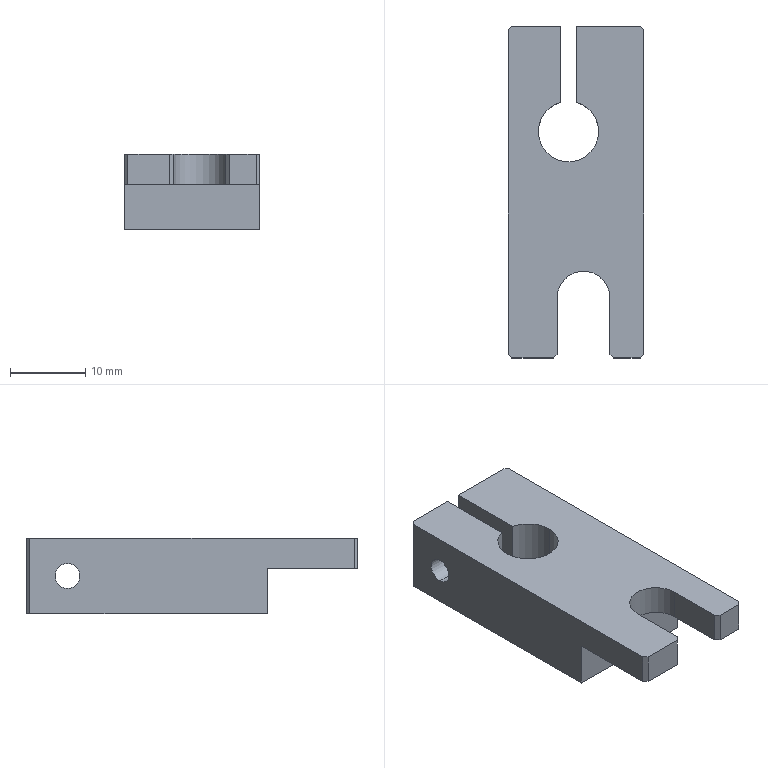Part | NX | features BREP 1 | 1 solid | 31 faces | box 18 x 44 x 10 mm | volume 5264 mm3 | plane 21 | cylinder 10 | commonest cylinder face diameters 8 x5 3.3 x2 4.8 x2 7 x1
STEP:
#1=CARTESIAN_POINT('',(6.,38.5,4.));
#2=VERTEX_POINT('',#1);
#3=CARTESIAN_POINT('',(6.,38.5,-4.));
#4=VERTEX_POINT('',#3);
#5=CARTESIAN_POINT('',(6.,38.5,0.));
#6=DIRECTION('',(1.,0.,0.));
#7=DIRECTION('',(0.,0.,-1.));
#8=AXIS2_PLACEMENT_3D('',#5,#6,#7);
#9=CIRCLE('',#8,4.);
#10=EDGE_CURVE('',#2,#4,#9,.T.);
#11=ORIENTED_EDGE('',*,*,#10,.F.);
#12=CARTESIAN_POINT('',(10.,38.5,4.));
#13=VERTEX_POINT('',#12);
#14=CARTESIAN_POINT('',(10.,38.5,4.));
#15=DIRECTION('',(1.,0.,0.));
#16=VECTOR('',#15,1000.);
#17=LINE('',#14,#16);
#18=EDGE_CURVE('',#2,#13,#17,.T.);
#19=ORIENTED_EDGE('',*,*,#18,.T.);
#20=CARTESIAN_POINT('',(10.,38.5,-4.));
#21=VERTEX_POINT('',#20);
#22=CARTESIAN_POINT('',(10.,38.5,0.));
#23=DIRECTION('',(1.,0.,0.));
#24=DIRECTION('',(0.,0.,-1.));
#25=AXIS2_PLACEMENT_3D('',#22,#23,#24);
#26=CIRCLE('',#25,4.);
#27=EDGE_CURVE('',#13,#21,#26,.T.);
#28=ORIENTED_EDGE('',*,*,#27,.T.);
#29=CARTESIAN_POINT('',(10.,38.5,-4.));
#30=DIRECTION('',(1.,0.,0.));
#31=VECTOR('',#30,1000.);
#32=LINE('',#29,#31);
#33=EDGE_CURVE('',#4,#21,#32,.T.);
#34=ORIENTED_EDGE('',*,*,#33,.F.);
#35=EDGE_LOOP('',(#11,#19,#28,#34));
#36=FACE_BOUND('',#35,.T.);
#37=CARTESIAN_POINT('',(10.,38.5,0.));
#38=DIRECTION('',(1.,0.,0.));
#39=DIRECTION('',(0.,0.,-1.));
#40=AXIS2_PLACEMENT_3D('',#37,#38,#39);
#41=CYLINDRICAL_SURFACE('',#40,4.);
#42=ADVANCED_FACE('',(#36),#41,.F.);
#43=CARTESIAN_POINT('',(1.,38.5,-2.4));
#44=VERTEX_POINT('',#43);
#45=CARTESIAN_POINT('',(1.,38.5,2.4));
#46=VERTEX_POINT('',#45);
#47=CARTESIAN_POINT('',(1.,38.5,0.));
#48=DIRECTION('',(-1.,0.,0.));
#49=DIRECTION('',(0.,0.,1.));
#50=AXIS2_PLACEMENT_3D('',#47,#48,#49);
#51=CIRCLE('',#50,2.4);
#52=EDGE_CURVE('',#44,#46,#51,.T.);
#53=ORIENTED_EDGE('',*,*,#52,.T.);
#54=CARTESIAN_POINT('',(6.,38.5,2.4));
#55=VERTEX_POINT('',#54);
#56=CARTESIAN_POINT('',(10.,38.5,2.4));
#57=DIRECTION('',(1.,0.,0.));
#58=VECTOR('',#57,1000.);
#59=LINE('',#56,#58);
#60=EDGE_CURVE('',#46,#55,#59,.T.);
#61=ORIENTED_EDGE('',*,*,#60,.T.);
#62=CARTESIAN_POINT('',(6.,38.5,-2.4));
#63=VERTEX_POINT('',#62);
#64=CARTESIAN_POINT('',(6.,38.5,0.));
#65=DIRECTION('',(1.,0.,0.));
#66=DIRECTION('',(0.,0.,-1.));
#67=AXIS2_PLACEMENT_3D('',#64,#65,#66);
#68=CIRCLE('',#67,2.4);
#69=EDGE_CURVE('',#55,#63,#68,.T.);
#70=ORIENTED_EDGE('',*,*,#69,.T.);
#71=CARTESIAN_POINT('',(10.,38.5,-2.4));
#72=DIRECTION('',(1.,0.,0.));
#73=VECTOR('',#72,1000.);
#74=LINE('',#71,#73);
#75=EDGE_CURVE('',#44,#63,#74,.T.);
#76=ORIENTED_EDGE('',*,*,#75,.F.);
#77=EDGE_LOOP('',(#53,#61,#70,#76));
#78=FACE_BOUND('',#77,.T.);
#79=CARTESIAN_POINT('',(10.,38.5,0.));
#80=DIRECTION('',(1.,0.,0.));
#81=DIRECTION('',(0.,0.,-1.));
#82=AXIS2_PLACEMENT_3D('',#79,#80,#81);
#83=CYLINDRICAL_SURFACE('',#82,2.4);
#84=ADVANCED_FACE('',(#78),#83,.F.);
#85=CARTESIAN_POINT('',(-8.,38.5,1.65));
#86=VERTEX_POINT('',#85);
#87=CARTESIAN_POINT('',(-8.,38.5,-1.65));
#88=VERTEX_POINT('',#87);
#89=CARTESIAN_POINT('',(-8.,38.5,0.));
#90=DIRECTION('',(1.,0.,0.));
#91=DIRECTION('',(0.,0.,-1.));
#92=AXIS2_PLACEMENT_3D('',#89,#90,#91);
#93=CIRCLE('',#92,1.65);
#94=EDGE_CURVE('',#86,#88,#93,.T.);
#95=ORIENTED_EDGE('',*,*,#94,.F.);
#96=CARTESIAN_POINT('',(-1.,38.5,1.65));
#97=VERTEX_POINT('',#96);
#98=CARTESIAN_POINT('',(-1.,38.5,1.65));
#99=DIRECTION('',(1.,0.,0.));
#100=VECTOR('',#99,1000.);
#101=LINE('',#98,#100);
#102=EDGE_CURVE('',#86,#97,#101,.T.);
#103=ORIENTED_EDGE('',*,*,#102,.T.);
#104=CARTESIAN_POINT('',(-1.,38.5,-1.65));
#105=VERTEX_POINT('',#104);
#106=CARTESIAN_POINT('',(-1.,38.5,0.));
#107=DIRECTION('',(1.,0.,0.));
#108=DIRECTION('',(0.,0.,-1.));
#109=AXIS2_PLACEMENT_3D('',#106,#107,#108);
#110=CIRCLE('',#109,1.65);
#111=EDGE_CURVE('',#97,#105,#110,.T.);
#112=ORIENTED_EDGE('',*,*,#111,.T.);
#113=CARTESIAN_POINT('',(-1.,38.5,-1.65));
#114=DIRECTION('',(1.,0.,0.));
#115=VECTOR('',#114,1000.);
#116=LINE('',#113,#115);
#117=EDGE_CURVE('',#88,#105,#116,.T.);
#118=ORIENTED_EDGE('',*,*,#117,.F.);
#119=EDGE_LOOP('',(#95,#103,#112,#118));
#120=FACE_BOUND('',#119,.T.);
#121=CARTESIAN_POINT('',(-1.,38.5,0.));
#122=DIRECTION('',(1.,0.,0.));
#123=DIRECTION('',(0.,0.,-1.));
#124=AXIS2_PLACEMENT_3D('',#121,#122,#123);
#125=CYLINDRICAL_SURFACE('',#124,1.65);
#126=ADVANCED_FACE('',(#120),#125,.F.);
#127=CARTESIAN_POINT('',(-4.,30.,5.));
#128=VERTEX_POINT('',#127);
#129=CARTESIAN_POINT('',(4.,30.,5.));
#130=VERTEX_POINT('',#129);
#131=CARTESIAN_POINT('',(0.,30.,5.));
#132=DIRECTION('',(0.,0.,1.));
#133=DIRECTION('',(1.,0.,0.));
#134=AXIS2_PLACEMENT_3D('',#131,#132,#133);
#135=CIRCLE('',#134,4.);
#136=EDGE_CURVE('',#128,#130,#135,.T.);
#137=ORIENTED_EDGE('',*,*,#136,.T.);
#138=CARTESIAN_POINT('',(4.,30.,-5.));
#139=VERTEX_POINT('',#138);
#140=CARTESIAN_POINT('',(4.,30.,5.));
#141=DIRECTION('',(0.,0.,-1.));
#142=VECTOR('',#141,1000.);
#143=LINE('',#140,#142);
#144=EDGE_CURVE('',#130,#139,#143,.T.);
#145=ORIENTED_EDGE('',*,*,#144,.T.);
#146=CARTESIAN_POINT('',(-4.,30.,-5.));
#147=VERTEX_POINT('',#146);
#148=CARTESIAN_POINT('',(0.,30.,-5.));
#149=DIRECTION('',(0.,0.,1.));
#150=DIRECTION('',(1.,0.,0.));
#151=AXIS2_PLACEMENT_3D('',#148,#149,#150);
#152=CIRCLE('',#151,4.);
#153=EDGE_CURVE('',#147,#139,#152,.T.);
#154=ORIENTED_EDGE('',*,*,#153,.F.);
#155=CARTESIAN_POINT('',(-4.,30.,5.));
#156=DIRECTION('',(0.,0.,-1.));
#157=VECTOR('',#156,1000.);
#158=LINE('',#155,#157);
#159=EDGE_CURVE('',#128,#147,#158,.T.);
#160=ORIENTED_EDGE('',*,*,#159,.F.);
#161=EDGE_LOOP('',(#137,#145,#154,#160));
#162=FACE_BOUND('',#161,.T.);
#163=CARTESIAN_POINT('',(0.,30.,5.));
#164=DIRECTION('',(0.,0.,-1.));
#165=DIRECTION('',(-1.,0.,0.));
#166=AXIS2_PLACEMENT_3D('',#163,#164,#165);
#167=CYLINDRICAL_SURFACE('',#166,4.);
#168=ADVANCED_FACE('',(#162),#167,.F.);
#169=CARTESIAN_POINT('',(-1.,33.873,5.));
#170=VERTEX_POINT('',#169);
#171=CARTESIAN_POINT('',(0.,30.,5.));
#172=DIRECTION('',(0.,0.,1.));
#173=DIRECTION('',(1.,0.,0.));
#174=AXIS2_PLACEMENT_3D('',#171,#172,#173);
#175=CIRCLE('',#174,4.);
#176=EDGE_CURVE('',#170,#128,#175,.T.);
#177=ORIENTED_EDGE('',*,*,#176,.T.);
#178=ORIENTED_EDGE('',*,*,#159,.T.);
#179=CARTESIAN_POINT('',(-1.,33.873,-5.));
#180=VERTEX_POINT('',#179);
#181=CARTESIAN_POINT('',(0.,30.,-5.));
#182=DIRECTION('',(0.,0.,1.));
#183=DIRECTION('',(1.,0.,0.));
#184=AXIS2_PLACEMENT_3D('',#181,#182,#183);
#185=CIRCLE('',#184,4.);
#186=EDGE_CURVE('',#180,#147,#185,.T.);
#187=ORIENTED_EDGE('',*,*,#186,.F.);
#188=CARTESIAN_POINT('',(-1.,33.873,5.));
#189=DIRECTION('',(0.,0.,1.));
#190=VECTOR('',#189,1000.);
#191=LINE('',#188,#190);
#192=EDGE_CURVE('',#180,#170,#191,.T.);
#193=ORIENTED_EDGE('',*,*,#192,.T.);
#194=EDGE_LOOP('',(#177,#178,#187,#193));
#195=FACE_BOUND('',#194,.T.);
#196=CARTESIAN_POINT('',(0.,30.,5.));
#197=DIRECTION('',(0.,0.,-1.));
#198=DIRECTION('',(-1.,0.,0.));
#199=AXIS2_PLACEMENT_3D('',#196,#197,#198);
#200=CYLINDRICAL_SURFACE('',#199,4.);
#201=ADVANCED_FACE('',(#195),#200,.F.);
#202=CARTESIAN_POINT('',(6.,0.,1.));
#203=VERTEX_POINT('',#202);
#204=CARTESIAN_POINT('',(9.5,0.,1.));
#205=VERTEX_POINT('',#204);
#206=CARTESIAN_POINT('',(-8.,0.,1.));
#207=DIRECTION('',(1.,0.,0.));
#208=VECTOR('',#207,1000.);
#209=LINE('',#206,#208);
#210=EDGE_CURVE('',#203,#205,#209,.T.);
#211=ORIENTED_EDGE('',*,*,#210,.T.);
#212=CARTESIAN_POINT('',(9.5,0.,5.));
#213=VERTEX_POINT('',#212);
#214=CARTESIAN_POINT('',(9.5,0.,5.));
#215=DIRECTION('',(0.,0.,1.));
#216=VECTOR('',#215,1000.);
#217=LINE('',#214,#216);
#218=EDGE_CURVE('',#205,#213,#217,.T.);
#219=ORIENTED_EDGE('',*,*,#218,.T.);
#220=CARTESIAN_POINT('',(6.,0.,5.));
#221=VERTEX_POINT('',#220);
#222=CARTESIAN_POINT('',(-8.,0.,5.));
#223=DIRECTION('',(1.,0.,0.));
#224=VECTOR('',#223,1000.);
#225=LINE('',#222,#224);
#226=EDGE_CURVE('',#221,#213,#225,.T.);
#227=ORIENTED_EDGE('',*,*,#226,.F.);
#228=CARTESIAN_POINT('',(6.,0.,5.));
#229=DIRECTION('',(0.,0.,-1.));
#230=VECTOR('',#229,1000.);
#231=LINE('',#228,#230);
#232=EDGE_CURVE('',#221,#203,#231,.T.);
#233=ORIENTED_EDGE('',*,*,#232,.T.);
#234=EDGE_LOOP('',(#211,#219,#227,#233));
#235=FACE_BOUND('',#234,.T.);
#236=CARTESIAN_POINT('',(-8.,0.,5.));
#237=DIRECTION('',(0.,1.,0.));
#238=DIRECTION('',(1.,0.,0.));
#239=AXIS2_PLACEMENT_3D('',#236,#237,#238);
#240=PLANE('',#239);
#241=ADVANCED_FACE('',(#235),#240,.F.);
#242=CARTESIAN_POINT('',(-1.,44.,5.));
#243=VERTEX_POINT('',#242);
#244=CARTESIAN_POINT('',(-7.5,44.,5.));
#245=VERTEX_POINT('',#244);
#246=CARTESIAN_POINT('',(10.,44.,5.));
#247=DIRECTION('',(-1.,0.,0.));
#248=VECTOR('',#247,1000.);
#249=LINE('',#246,#248);
#250=EDGE_CURVE('',#243,#245,#249,.T.);
#251=ORIENTED_EDGE('',*,*,#250,.T.);
#252=CARTESIAN_POINT('',(-8.,43.5,5.));
#253=VERTEX_POINT('',#252);
#254=CARTESIAN_POINT('',(1.25,52.75,5.));
#255=DIRECTION('',(-0.7071,-0.7071,0.));
#256=VECTOR('',#255,1000.);
#257=LINE('',#254,#256);
#258=EDGE_CURVE('',#245,#253,#257,.T.);
#259=ORIENTED_EDGE('',*,*,#258,.T.);
#260=CARTESIAN_POINT('',(-8.,0.5,5.));
#261=VERTEX_POINT('',#260);
#262=CARTESIAN_POINT('',(-8.,0.,5.));
#263=DIRECTION('',(0.,-1.,0.));
#264=VECTOR('',#263,1000.);
#265=LINE('',#262,#264);
#266=EDGE_CURVE('',#253,#261,#265,.T.);
#267=ORIENTED_EDGE('',*,*,#266,.T.);
#268=CARTESIAN_POINT('',(-7.5,0.,5.));
#269=VERTEX_POINT('',#268);
#270=CARTESIAN_POINT('',(-20.75,13.25,5.));
#271=DIRECTION('',(0.7071,-0.7071,0.));
#272=VECTOR('',#271,1000.);
#273=LINE('',#270,#272);
#274=EDGE_CURVE('',#261,#269,#273,.T.);
#275=ORIENTED_EDGE('',*,*,#274,.T.);
#276=CARTESIAN_POINT('',(-2.,0.,5.));
#277=VERTEX_POINT('',#276);
#278=CARTESIAN_POINT('',(-8.,0.,5.));
#279=DIRECTION('',(1.,0.,0.));
#280=VECTOR('',#279,1000.);
#281=LINE('',#278,#280);
#282=EDGE_CURVE('',#269,#277,#281,.T.);
#283=ORIENTED_EDGE('',*,*,#282,.T.);
#284=CARTESIAN_POINT('',(-1.5,0.5,5.));
#285=VERTEX_POINT('',#284);
#286=CARTESIAN_POINT('',(26.,28.,5.));
#287=DIRECTION('',(0.7071,0.7071,0.));
#288=VECTOR('',#287,1000.);
#289=LINE('',#286,#288);
#290=EDGE_CURVE('',#277,#285,#289,.T.);
#291=ORIENTED_EDGE('',*,*,#290,.T.);
#292=CARTESIAN_POINT('',(-1.5,8.,5.));
#293=VERTEX_POINT('',#292);
#294=CARTESIAN_POINT('',(-1.5,8.,5.));
#295=DIRECTION('',(0.,1.,0.));
#296=VECTOR('',#295,1000.);
#297=LINE('',#294,#296);
#298=EDGE_CURVE('',#285,#293,#297,.T.);
#299=ORIENTED_EDGE('',*,*,#298,.T.);
#300=CARTESIAN_POINT('',(5.5,8.,5.));
#301=VERTEX_POINT('',#300);
#302=CARTESIAN_POINT('',(2.,8.,5.));
#303=DIRECTION('',(0.,0.,-1.));
#304=DIRECTION('',(-1.,0.,0.));
#305=AXIS2_PLACEMENT_3D('',#302,#303,#304);
#306=CIRCLE('',#305,3.5);
#307=EDGE_CURVE('',#293,#301,#306,.T.);
#308=ORIENTED_EDGE('',*,*,#307,.T.);
#309=CARTESIAN_POINT('',(5.5,0.5,5.));
#310=VERTEX_POINT('',#309);
#311=CARTESIAN_POINT('',(5.5,8.,5.));
#312=DIRECTION('',(0.,-1.,0.));
#313=VECTOR('',#312,1000.);
#314=LINE('',#311,#313);
#315=EDGE_CURVE('',#301,#310,#314,.T.);
#316=ORIENTED_EDGE('',*,*,#315,.T.);
#317=CARTESIAN_POINT('',(-14.,20.,5.));
#318=DIRECTION('',(0.7071,-0.7071,0.));
#319=VECTOR('',#318,1000.);
#320=LINE('',#317,#319);
#321=EDGE_CURVE('',#310,#221,#320,.T.);
#322=ORIENTED_EDGE('',*,*,#321,.T.);
#323=ORIENTED_EDGE('',*,*,#226,.T.);
#324=CARTESIAN_POINT('',(10.,0.5,5.));
#325=VERTEX_POINT('',#324);
#326=CARTESIAN_POINT('',(31.75,22.25,5.));
#327=DIRECTION('',(0.7071,0.7071,0.));
#328=VECTOR('',#327,1000.);
#329=LINE('',#326,#328);
#330=EDGE_CURVE('',#213,#325,#329,.T.);
#331=ORIENTED_EDGE('',*,*,#330,.T.);
#332=CARTESIAN_POINT('',(10.,43.5,5.));
#333=VERTEX_POINT('',#332);
#334=CARTESIAN_POINT('',(10.,0.,5.));
#335=DIRECTION('',(0.,1.,0.));
#336=VECTOR('',#335,1000.);
#337=LINE('',#334,#336);
#338=EDGE_CURVE('',#325,#333,#337,.T.);
#339=ORIENTED_EDGE('',*,*,#338,.T.);
#340=CARTESIAN_POINT('',(9.5,44.,5.));
#341=VERTEX_POINT('',#340);
#342=CARTESIAN_POINT('',(9.75,43.75,5.));
#343=DIRECTION('',(-0.7071,0.7071,0.));
#344=VECTOR('',#343,1000.);
#345=LINE('',#342,#344);
#346=EDGE_CURVE('',#333,#341,#345,.T.);
#347=ORIENTED_EDGE('',*,*,#346,.T.);
#348=CARTESIAN_POINT('',(1.,44.,5.));
#349=VERTEX_POINT('',#348);
#350=CARTESIAN_POINT('',(10.,44.,5.));
#351=DIRECTION('',(-1.,0.,0.));
#352=VECTOR('',#351,1000.);
#353=LINE('',#350,#352);
#354=EDGE_CURVE('',#341,#349,#353,.T.);
#355=ORIENTED_EDGE('',*,*,#354,.T.);
#356=CARTESIAN_POINT('',(1.,33.873,5.));
#357=VERTEX_POINT('',#356);
#358=CARTESIAN_POINT('',(1.,44.,5.));
#359=DIRECTION('',(0.,-1.,0.));
#360=VECTOR('',#359,1000.);
#361=LINE('',#358,#360);
#362=EDGE_CURVE('',#349,#357,#361,.T.);
#363=ORIENTED_EDGE('',*,*,#362,.T.);
#364=CARTESIAN_POINT('',(0.,30.,5.));
#365=DIRECTION('',(0.,0.,1.));
#366=DIRECTION('',(1.,0.,0.));
#367=AXIS2_PLACEMENT_3D('',#364,#365,#366);
#368=CIRCLE('',#367,4.);
#369=EDGE_CURVE('',#130,#357,#368,.T.);
#370=ORIENTED_EDGE('',*,*,#369,.F.);
#371=ORIENTED_EDGE('',*,*,#136,.F.);
#372=ORIENTED_EDGE('',*,*,#176,.F.);
#373=CARTESIAN_POINT('',(-1.,44.,5.));
#374=DIRECTION('',(0.,1.,0.));
#375=VECTOR('',#374,1000.);
#376=LINE('',#373,#375);
#377=EDGE_CURVE('',#170,#243,#376,.T.);
#378=ORIENTED_EDGE('',*,*,#377,.T.);
#379=EDGE_LOOP('',(#251,#259,#267,#275,#283,#291,#299,#308,#316,#322,#323,#331,#339,#347,#355,#363,#370,#371,#372,#378));
#380=FACE_BOUND('',#379,.T.);
#381=CARTESIAN_POINT('',(10.,44.,5.));
#382=DIRECTION('',(0.,0.,1.));
#383=DIRECTION('',(1.,0.,0.));
#384=AXIS2_PLACEMENT_3D('',#381,#382,#383);
#385=PLANE('',#384);
#386=ADVANCED_FACE('',(#380),#385,.T.);
#387=CARTESIAN_POINT('',(-1.,44.,-5.));
#388=VERTEX_POINT('',#387);
#389=CARTESIAN_POINT('',(-7.5,44.,-5.));
#390=VERTEX_POINT('',#389);
#391=CARTESIAN_POINT('',(10.,44.,-5.));
#392=DIRECTION('',(-1.,0.,0.));
#393=VECTOR('',#392,1000.);
#394=LINE('',#391,#393);
#395=EDGE_CURVE('',#388,#390,#394,.T.);
#396=ORIENTED_EDGE('',*,*,#395,.T.);
#397=CARTESIAN_POINT('',(-7.5,44.,5.));
#398=DIRECTION('',(0.,0.,1.));
#399=VECTOR('',#398,1000.);
#400=LINE('',#397,#399);
#401=EDGE_CURVE('',#390,#245,#400,.T.);
#402=ORIENTED_EDGE('',*,*,#401,.T.);
#403=ORIENTED_EDGE('',*,*,#250,.F.);
#404=CARTESIAN_POINT('',(-1.,44.,6.));
#405=DIRECTION('',(0.,0.,-1.));
#406=VECTOR('',#405,1000.);
#407=LINE('',#404,#406);
#408=EDGE_CURVE('',#243,#388,#407,.T.);
#409=ORIENTED_EDGE('',*,*,#408,.T.);
#410=EDGE_LOOP('',(#396,#402,#403,#409));
#411=FACE_BOUND('',#410,.T.);
#412=CARTESIAN_POINT('',(10.,44.,5.));
#413=DIRECTION('',(0.,-1.,0.));
#414=DIRECTION('',(0.,0.,-1.));
#415=AXIS2_PLACEMENT_3D('',#412,#413,#414);
#416=PLANE('',#415);
#417=ADVANCED_FACE('',(#411),#416,.F.);
#418=ORIENTED_EDGE('',*,*,#354,.F.);
#419=CARTESIAN_POINT('',(9.5,44.,-5.));
#420=VERTEX_POINT('',#419);
#421=CARTESIAN_POINT('',(9.5,44.,5.));
#422=DIRECTION('',(0.,0.,-1.));
#423=VECTOR('',#422,1000.);
#424=LINE('',#421,#423);
#425=EDGE_CURVE('',#341,#420,#424,.T.);
#426=ORIENTED_EDGE('',*,*,#425,.T.);
#427=CARTESIAN_POINT('',(1.,44.,-5.));
#428=VERTEX_POINT('',#427);
#429=CARTESIAN_POINT('',(10.,44.,-5.));
#430=DIRECTION('',(-1.,0.,0.));
#431=VECTOR('',#430,1000.);
#432=LINE('',#429,#431);
#433=EDGE_CURVE('',#420,#428,#432,.T.);
#434=ORIENTED_EDGE('',*,*,#433,.T.);
#435=CARTESIAN_POINT('',(1.,44.,6.));
#436=DIRECTION('',(0.,0.,-1.));
#437=VECTOR('',#436,1000.);
#438=LINE('',#435,#437);
#439=EDGE_CURVE('',#349,#428,#438,.T.);
#440=ORIENTED_EDGE('',*,*,#439,.F.);
#441=EDGE_LOOP('',(#418,#426,#434,#440));
#442=FACE_BOUND('',#441,.T.);
#443=CARTESIAN_POINT('',(10.,44.,5.));
#444=DIRECTION('',(0.,-1.,0.));
#445=DIRECTION('',(0.,0.,-1.));
#446=AXIS2_PLACEMENT_3D('',#443,#444,#445);
#447=PLANE('',#446);
#448=ADVANCED_FACE('',(#442),#447,.F.);
#449=ORIENTED_EDGE('',*,*,#144,.F.);
#450=ORIENTED_EDGE('',*,*,#369,.T.);
#451=CARTESIAN_POINT('',(1.,33.873,-5.));
#452=VERTEX_POINT('',#451);
#453=CARTESIAN_POINT('',(1.,33.873,5.));
#454=DIRECTION('',(0.,0.,-1.));
#455=VECTOR('',#454,1000.);
#456=LINE('',#453,#455);
#457=EDGE_CURVE('',#357,#452,#456,.T.);
#458=ORIENTED_EDGE('',*,*,#457,.T.);
#459=CARTESIAN_POINT('',(0.,30.,-5.));
#460=DIRECTION('',(0.,0.,1.));
#461=DIRECTION('',(1.,0.,0.));
#462=AXIS2_PLACEMENT_3D('',#459,#460,#461);
#463=CIRCLE('',#462,4.);
#464=EDGE_CURVE('',#139,#452,#463,.T.);
#465=ORIENTED_EDGE('',*,*,#464,.F.);
#466=EDGE_LOOP('',(#449,#450,#458,#465));
#467=FACE_BOUND('',#466,.T.);
#468=CARTESIAN_POINT('',(0.,30.,5.));
#469=DIRECTION('',(0.,0.,-1.));
#470=DIRECTION('',(-1.,0.,0.));
#471=AXIS2_PLACEMENT_3D('',#468,#469,#470);
#472=CYLINDRICAL_SURFACE('',#471,4.);
#473=ADVANCED_FACE('',(#467),#472,.F.);
#474=CARTESIAN_POINT('',(-8.,43.5,-5.));
#475=VERTEX_POINT('',#474);
#476=CARTESIAN_POINT('',(-8.,12.,-5.));
#477=VERTEX_POINT('',#476);
#478=CARTESIAN_POINT('',(-8.,0.,-5.));
#479=DIRECTION('',(0.,-1.,0.));
#480=VECTOR('',#479,1000.);
#481=LINE('',#478,#480);
#482=EDGE_CURVE('',#475,#477,#481,.T.);
#483=ORIENTED_EDGE('',*,*,#482,.F.);
#484=CARTESIAN_POINT('',(-8.,43.5,-5.));
#485=DIRECTION('',(0.7071,0.7071,0.));
#486=VECTOR('',#485,1000.);
#487=LINE('',#484,#486);
#488=EDGE_CURVE('',#475,#390,#487,.T.);
#489=ORIENTED_EDGE('',*,*,#488,.T.);
#490=ORIENTED_EDGE('',*,*,#395,.F.);
#491=CARTESIAN_POINT('',(-1.,44.,-5.));
#492=DIRECTION('',(0.,1.,0.));
#493=VECTOR('',#492,1000.);
#494=LINE('',#491,#493);
#495=EDGE_CURVE('',#180,#388,#494,.T.);
#496=ORIENTED_EDGE('',*,*,#495,.F.);
#497=ORIENTED_EDGE('',*,*,#186,.T.);
#498=ORIENTED_EDGE('',*,*,#153,.T.);
#499=ORIENTED_EDGE('',*,*,#464,.T.);
#500=CARTESIAN_POINT('',(1.,44.,-5.));
#501=DIRECTION('',(0.,-1.,0.));
#502=VECTOR('',#501,1000.);
#503=LINE('',#500,#502);
#504=EDGE_CURVE('',#428,#452,#503,.T.);
#505=ORIENTED_EDGE('',*,*,#504,.F.);
#506=ORIENTED_EDGE('',*,*,#433,.F.);
#507=CARTESIAN_POINT('',(10.,43.5,-5.));
#508=VERTEX_POINT('',#507);
#509=CARTESIAN_POINT('',(9.5,44.,-5.));
#510=DIRECTION('',(0.7071,-0.7071,0.));
#511=VECTOR('',#510,1000.);
#512=LINE('',#509,#511);
#513=EDGE_CURVE('',#420,#508,#512,.T.);
#514=ORIENTED_EDGE('',*,*,#513,.T.);
#515=CARTESIAN_POINT('',(10.,12.,-5.));
#516=VERTEX_POINT('',#515);
#517=CARTESIAN_POINT('',(10.,0.,-5.));
#518=DIRECTION('',(0.,1.,0.));
#519=VECTOR('',#518,1000.);
#520=LINE('',#517,#519);
#521=EDGE_CURVE('',#516,#508,#520,.T.);
#522=ORIENTED_EDGE('',*,*,#521,.F.);
#523=CARTESIAN_POINT('',(-12.792,12.,-5.));
#524=DIRECTION('',(1.,0.,0.));
#525=VECTOR('',#524,1000.);
#526=LINE('',#523,#525);
#527=EDGE_CURVE('',#477,#516,#526,.T.);
#528=ORIENTED_EDGE('',*,*,#527,.F.);
#529=EDGE_LOOP('',(#483,#489,#490,#496,#497,#498,#499,#505,#506,#514,#522,#528));
#530=FACE_BOUND('',#529,.T.);
#531=CARTESIAN_POINT('',(10.,44.,-5.));
#532=DIRECTION('',(0.,0.,1.));
#533=DIRECTION('',(1.,0.,0.));
#534=AXIS2_PLACEMENT_3D('',#531,#532,#533);
#535=PLANE('',#534);
#536=ADVANCED_FACE('',(#530),#535,.F.);
#537=ORIENTED_EDGE('',*,*,#521,.T.);
#538=CARTESIAN_POINT('',(10.,43.5,5.));
#539=DIRECTION('',(0.,0.,1.));
#540=VECTOR('',#539,1000.);
#541=LINE('',#538,#540);
#542=EDGE_CURVE('',#508,#333,#541,.T.);
#543=ORIENTED_EDGE('',*,*,#542,.T.);
#544=ORIENTED_EDGE('',*,*,#338,.F.);
#545=CARTESIAN_POINT('',(10.,0.5,1.));
#546=VERTEX_POINT('',#545);
#547=CARTESIAN_POINT('',(10.,0.5,5.));
#548=DIRECTION('',(0.,0.,-1.));
#549=VECTOR('',#548,1000.);
#550=LINE('',#547,#549);
#551=EDGE_CURVE('',#325,#546,#550,.T.);
#552=ORIENTED_EDGE('',*,*,#551,.T.);
#553=CARTESIAN_POINT('',(10.,12.,1.));
#554=VERTEX_POINT('',#553);
#555=CARTESIAN_POINT('',(10.,0.,1.));
#556=DIRECTION('',(0.,1.,0.));
#557=VECTOR('',#556,1000.);
#558=LINE('',#555,#557);
#559=EDGE_CURVE('',#546,#554,#558,.T.);
#560=ORIENTED_EDGE('',*,*,#559,.T.);
#561=CARTESIAN_POINT('',(10.,12.,5.));
#562=DIRECTION('',(0.,0.,-1.));
#563=VECTOR('',#562,1000.);
#564=LINE('',#561,#563);
#565=EDGE_CURVE('',#554,#516,#564,.T.);
#566=ORIENTED_EDGE('',*,*,#565,.T.);
#567=EDGE_LOOP('',(#537,#543,#544,#552,#560,#566));
#568=FACE_BOUND('',#567,.T.);
#569=CARTESIAN_POINT('',(10.,38.5,0.));
#570=DIRECTION('',(1.,0.,0.));
#571=DIRECTION('',(0.,0.,-1.));
#572=AXIS2_PLACEMENT_3D('',#569,#570,#571);
#573=CIRCLE('',#572,4.);
#574=EDGE_CURVE('',#21,#13,#573,.T.);
#575=ORIENTED_EDGE('',*,*,#574,.F.);
#576=ORIENTED_EDGE('',*,*,#27,.F.);
#577=EDGE_LOOP('',(#575,#576));
#578=FACE_BOUND('',#577,.T.);
#579=CARTESIAN_POINT('',(10.,0.,5.));
#580=DIRECTION('',(-1.,0.,0.));
#581=DIRECTION('',(0.,0.,1.));
#582=AXIS2_PLACEMENT_3D('',#579,#580,#581);
#583=PLANE('',#582);
#584=ADVANCED_FACE('',(#568,#578),#583,.F.);
#585=ORIENTED_EDGE('',*,*,#266,.F.);
#586=CARTESIAN_POINT('',(-8.,43.5,5.));
#587=DIRECTION('',(0.,0.,-1.));
#588=VECTOR('',#587,1000.);
#589=LINE('',#586,#588);
#590=EDGE_CURVE('',#253,#475,#589,.T.);
#591=ORIENTED_EDGE('',*,*,#590,.T.);
#592=ORIENTED_EDGE('',*,*,#482,.T.);
#593=CARTESIAN_POINT('',(-8.,12.,1.));
#594=VERTEX_POINT('',#593);
#595=CARTESIAN_POINT('',(-8.,12.,5.));
#596=DIRECTION('',(0.,0.,1.));
#597=VECTOR('',#596,1000.);
#598=LINE('',#595,#597);
#599=EDGE_CURVE('',#477,#594,#598,.T.);
#600=ORIENTED_EDGE('',*,*,#599,.T.);
#601=CARTESIAN_POINT('',(-8.,0.5,1.));
#602=VERTEX_POINT('',#601);
#603=CARTESIAN_POINT('',(-8.,0.,1.));
#604=DIRECTION('',(0.,-1.,0.));
#605=VECTOR('',#604,1000.);
#606=LINE('',#603,#605);
#607=EDGE_CURVE('',#594,#602,#606,.T.);
#608=ORIENTED_EDGE('',*,*,#607,.T.);
#609=CARTESIAN_POINT('',(-8.,0.5,5.));
#610=DIRECTION('',(0.,0.,1.));
#611=VECTOR('',#610,1000.);
#612=LINE('',#609,#611);
#613=EDGE_CURVE('',#602,#261,#612,.T.);
#614=ORIENTED_EDGE('',*,*,#613,.T.);
#615=EDGE_LOOP('',(#585,#591,#592,#600,#608,#614));
#616=FACE_BOUND('',#615,.T.);
#617=CARTESIAN_POINT('',(-8.,38.5,0.));
#618=DIRECTION('',(1.,0.,0.));
#619=DIRECTION('',(0.,0.,-1.));
#620=AXIS2_PLACEMENT_3D('',#617,#618,#619);
#621=CIRCLE('',#620,1.65);
#622=EDGE_CURVE('',#88,#86,#621,.T.);
#623=ORIENTED_EDGE('',*,*,#622,.T.);
#624=ORIENTED_EDGE('',*,*,#94,.T.);
#625=EDGE_LOOP('',(#623,#624));
#626=FACE_BOUND('',#625,.T.);
#627=CARTESIAN_POINT('',(-8.,0.,5.));
#628=DIRECTION('',(1.,0.,0.));
#629=DIRECTION('',(0.,1.,0.));
#630=AXIS2_PLACEMENT_3D('',#627,#628,#629);
#631=PLANE('',#630);
#632=ADVANCED_FACE('',(#616,#626),#631,.F.);
#633=ORIENTED_EDGE('',*,*,#282,.F.);
#634=CARTESIAN_POINT('',(-7.5,0.,1.));
#635=VERTEX_POINT('',#634);
#636=CARTESIAN_POINT('',(-7.5,0.,5.));
#637=DIRECTION('',(0.,0.,-1.));
#638=VECTOR('',#637,1000.);
#639=LINE('',#636,#638);
#640=EDGE_CURVE('',#269,#635,#639,.T.);
#641=ORIENTED_EDGE('',*,*,#640,.T.);
#642=CARTESIAN_POINT('',(-2.,0.,1.));
#643=VERTEX_POINT('',#642);
#644=CARTESIAN_POINT('',(-8.,0.,1.));
#645=DIRECTION('',(1.,0.,0.));
#646=VECTOR('',#645,1000.);
#647=LINE('',#644,#646);
#648=EDGE_CURVE('',#635,#643,#647,.T.);
#649=ORIENTED_EDGE('',*,*,#648,.T.);
#650=CARTESIAN_POINT('',(-2.,0.,5.));
#651=DIRECTION('',(0.,0.,1.));
#652=VECTOR('',#651,1000.);
#653=LINE('',#650,#652);
#654=EDGE_CURVE('',#643,#277,#653,.T.);
#655=ORIENTED_EDGE('',*,*,#654,.T.);
#656=EDGE_LOOP('',(#633,#641,#649,#655));
#657=FACE_BOUND('',#656,.T.);
#658=CARTESIAN_POINT('',(-8.,0.,5.));
#659=DIRECTION('',(0.,1.,0.));
#660=DIRECTION('',(1.,0.,0.));
#661=AXIS2_PLACEMENT_3D('',#658,#659,#660);
#662=PLANE('',#661);
#663=ADVANCED_FACE('',(#657),#662,.F.);
#664=ORIENTED_EDGE('',*,*,#439,.T.);
#665=ORIENTED_EDGE('',*,*,#504,.T.);
#666=ORIENTED_EDGE('',*,*,#457,.F.);
#667=ORIENTED_EDGE('',*,*,#362,.F.);
#668=EDGE_LOOP('',(#664,#665,#666,#667));
#669=FACE_BOUND('',#668,.T.);
#670=ORIENTED_EDGE('',*,*,#52,.F.);
#671=CARTESIAN_POINT('',(1.,38.5,0.));
#672=DIRECTION('',(-1.,0.,0.));
#673=DIRECTION('',(0.,0.,1.));
#674=AXIS2_PLACEMENT_3D('',#671,#672,#673);
#675=CIRCLE('',#674,2.4);
#676=EDGE_CURVE('',#46,#44,#675,.T.);
#677=ORIENTED_EDGE('',*,*,#676,.F.);
#678=EDGE_LOOP('',(#670,#677));
#679=FACE_BOUND('',#678,.T.);
#680=CARTESIAN_POINT('',(1.,28.,6.));
#681=DIRECTION('',(-1.,0.,0.));
#682=DIRECTION('',(0.,0.,1.));
#683=AXIS2_PLACEMENT_3D('',#680,#681,#682);
#684=PLANE('',#683);
#685=ADVANCED_FACE('',(#669,#679),#684,.T.);
#686=ORIENTED_EDGE('',*,*,#192,.F.);
#687=ORIENTED_EDGE('',*,*,#495,.T.);
#688=ORIENTED_EDGE('',*,*,#408,.F.);
#689=ORIENTED_EDGE('',*,*,#377,.F.);
#690=EDGE_LOOP('',(#686,#687,#688,#689));
#691=FACE_BOUND('',#690,.T.);
#692=CARTESIAN_POINT('',(-1.,38.5,0.));
#693=DIRECTION('',(1.,0.,0.));
#694=DIRECTION('',(0.,0.,-1.));
#695=AXIS2_PLACEMENT_3D('',#692,#693,#694);
#696=CIRCLE('',#695,1.65);
#697=EDGE_CURVE('',#105,#97,#696,.T.);
#698=ORIENTED_EDGE('',*,*,#697,.F.);
#699=ORIENTED_EDGE('',*,*,#111,.F.);
#700=EDGE_LOOP('',(#698,#699));
#701=FACE_BOUND('',#700,.T.);
#702=CARTESIAN_POINT('',(-1.,44.,6.));
#703=DIRECTION('',(1.,0.,0.));
#704=DIRECTION('',(0.,1.,0.));
#705=AXIS2_PLACEMENT_3D('',#702,#703,#704);
#706=PLANE('',#705);
#707=ADVANCED_FACE('',(#691,#701),#706,.T.);
#708=CARTESIAN_POINT('',(-12.792,12.,1.));
#709=DIRECTION('',(1.,0.,0.));
#710=VECTOR('',#709,1000.);
#711=LINE('',#708,#710);
#712=EDGE_CURVE('',#594,#554,#711,.T.);
#713=ORIENTED_EDGE('',*,*,#712,.F.);
#714=ORIENTED_EDGE('',*,*,#599,.F.);
#715=ORIENTED_EDGE('',*,*,#527,.T.);
#716=ORIENTED_EDGE('',*,*,#565,.F.);
#717=EDGE_LOOP('',(#713,#714,#715,#716));
#718=FACE_BOUND('',#717,.T.);
#719=CARTESIAN_POINT('',(-12.792,12.,1.));
#720=DIRECTION('',(0.,1.,0.));
#721=DIRECTION('',(1.,0.,0.));
#722=AXIS2_PLACEMENT_3D('',#719,#720,#721);
#723=PLANE('',#722);
#724=ADVANCED_FACE('',(#718),#723,.F.);
#725=ORIENTED_EDGE('',*,*,#559,.F.);
#726=CARTESIAN_POINT('',(10.,0.5,1.));
#727=DIRECTION('',(-0.7071,-0.7071,0.));
#728=VECTOR('',#727,1000.);
#729=LINE('',#726,#728);
#730=EDGE_CURVE('',#546,#205,#729,.T.);
#731=ORIENTED_EDGE('',*,*,#730,.T.);
#732=ORIENTED_EDGE('',*,*,#210,.F.);
#733=CARTESIAN_POINT('',(5.5,0.5,1.));
#734=VERTEX_POINT('',#733);
#735=CARTESIAN_POINT('',(6.,0.,1.));
#736=DIRECTION('',(-0.7071,0.7071,0.));
#737=VECTOR('',#736,1000.);
#738=LINE('',#735,#737);
#739=EDGE_CURVE('',#203,#734,#738,.T.);
#740=ORIENTED_EDGE('',*,*,#739,.T.);
#741=CARTESIAN_POINT('',(5.5,8.,1.));
#742=VERTEX_POINT('',#741);
#743=CARTESIAN_POINT('',(5.5,8.,1.));
#744=DIRECTION('',(0.,-1.,0.));
#745=VECTOR('',#744,1000.);
#746=LINE('',#743,#745);
#747=EDGE_CURVE('',#742,#734,#746,.T.);
#748=ORIENTED_EDGE('',*,*,#747,.F.);
#749=CARTESIAN_POINT('',(-1.5,8.,1.));
#750=VERTEX_POINT('',#749);
#751=CARTESIAN_POINT('',(2.,8.,1.));
#752=DIRECTION('',(0.,0.,-1.));
#753=DIRECTION('',(-1.,0.,0.));
#754=AXIS2_PLACEMENT_3D('',#751,#752,#753);
#755=CIRCLE('',#754,3.5);
#756=EDGE_CURVE('',#750,#742,#755,.T.);
#757=ORIENTED_EDGE('',*,*,#756,.F.);
#758=CARTESIAN_POINT('',(-1.5,0.5,1.));
#759=VERTEX_POINT('',#758);
#760=CARTESIAN_POINT('',(-1.5,-4.707,1.));
#761=DIRECTION('',(0.,-1.,0.));
#762=VECTOR('',#761,1000.);
#763=LINE('',#760,#762);
#764=EDGE_CURVE('',#750,#759,#763,.T.);
#765=ORIENTED_EDGE('',*,*,#764,.T.);
#766=CARTESIAN_POINT('',(-2.,0.,1.));
#767=DIRECTION('',(-0.7071,-0.7071,0.));
#768=VECTOR('',#767,1000.);
#769=LINE('',#766,#768);
#770=EDGE_CURVE('',#759,#643,#769,.T.);
#771=ORIENTED_EDGE('',*,*,#770,.T.);
#772=ORIENTED_EDGE('',*,*,#648,.F.);
#773=CARTESIAN_POINT('',(-7.5,0.,1.));
#774=DIRECTION('',(-0.7071,0.7071,0.));
#775=VECTOR('',#774,1000.);
#776=LINE('',#773,#775);
#777=EDGE_CURVE('',#635,#602,#776,.T.);
#778=ORIENTED_EDGE('',*,*,#777,.T.);
#779=ORIENTED_EDGE('',*,*,#607,.F.);
#780=ORIENTED_EDGE('',*,*,#712,.T.);
#781=EDGE_LOOP('',(#725,#731,#732,#740,#748,#757,#765,#771,#772,#778,#779,#780));
#782=FACE_BOUND('',#781,.T.);
#783=CARTESIAN_POINT('',(-12.792,-4.707,1.));
#784=DIRECTION('',(0.,0.,1.));
#785=DIRECTION('',(1.,0.,0.));
#786=AXIS2_PLACEMENT_3D('',#783,#784,#785);
#787=PLANE('',#786);
#788=ADVANCED_FACE('',(#782),#787,.F.);
#789=ORIENTED_EDGE('',*,*,#747,.T.);
#790=CARTESIAN_POINT('',(5.5,0.5,5.));
#791=DIRECTION('',(0.,0.,1.));
#792=VECTOR('',#791,1000.);
#793=LINE('',#790,#792);
#794=EDGE_CURVE('',#734,#310,#793,.T.);
#795=ORIENTED_EDGE('',*,*,#794,.T.);
#796=ORIENTED_EDGE('',*,*,#315,.F.);
#797=CARTESIAN_POINT('',(5.5,8.,5.));
#798=DIRECTION('',(0.,0.,-1.));
#799=VECTOR('',#798,1000.);
#800=LINE('',#797,#799);
#801=EDGE_CURVE('',#301,#742,#800,.T.);
#802=ORIENTED_EDGE('',*,*,#801,.T.);
#803=EDGE_LOOP('',(#789,#795,#796,#802));
#804=FACE_BOUND('',#803,.T.);
#805=CARTESIAN_POINT('',(5.5,8.,5.));
#806=DIRECTION('',(1.,0.,0.));
#807=DIRECTION('',(0.,1.,0.));
#808=AXIS2_PLACEMENT_3D('',#805,#806,#807);
#809=PLANE('',#808);
#810=ADVANCED_FACE('',(#804),#809,.F.);
#811=ORIENTED_EDGE('',*,*,#298,.F.);
#812=CARTESIAN_POINT('',(-1.5,0.5,5.));
#813=DIRECTION('',(0.,0.,-1.));
#814=VECTOR('',#813,1000.);
#815=LINE('',#812,#814);
#816=EDGE_CURVE('',#285,#759,#815,.T.);
#817=ORIENTED_EDGE('',*,*,#816,.T.);
#818=ORIENTED_EDGE('',*,*,#764,.F.);
#819=CARTESIAN_POINT('',(-1.5,8.,5.));
#820=DIRECTION('',(0.,0.,-1.));
#821=VECTOR('',#820,1000.);
#822=LINE('',#819,#821);
#823=EDGE_CURVE('',#293,#750,#822,.T.);
#824=ORIENTED_EDGE('',*,*,#823,.F.);
#825=EDGE_LOOP('',(#811,#817,#818,#824));
#826=FACE_BOUND('',#825,.T.);
#827=CARTESIAN_POINT('',(-1.5,8.,5.));
#828=DIRECTION('',(-1.,0.,0.));
#829=DIRECTION('',(0.,1.,0.));
#830=AXIS2_PLACEMENT_3D('',#827,#828,#829);
#831=PLANE('',#830);
#832=ADVANCED_FACE('',(#826),#831,.F.);
#833=ORIENTED_EDGE('',*,*,#756,.T.);
#834=ORIENTED_EDGE('',*,*,#801,.F.);
#835=ORIENTED_EDGE('',*,*,#307,.F.);
#836=ORIENTED_EDGE('',*,*,#823,.T.);
#837=EDGE_LOOP('',(#833,#834,#835,#836));
#838=FACE_BOUND('',#837,.T.);
#839=CARTESIAN_POINT('',(2.,8.,5.));
#840=DIRECTION('',(0.,0.,-1.));
#841=DIRECTION('',(-1.,0.,0.));
#842=AXIS2_PLACEMENT_3D('',#839,#840,#841);
#843=CYLINDRICAL_SURFACE('',#842,3.5);
#844=ADVANCED_FACE('',(#838),#843,.F.);
#845=ORIENTED_EDGE('',*,*,#102,.F.);
#846=ORIENTED_EDGE('',*,*,#622,.F.);
#847=ORIENTED_EDGE('',*,*,#117,.T.);
#848=ORIENTED_EDGE('',*,*,#697,.T.);
#849=EDGE_LOOP('',(#845,#846,#847,#848));
#850=FACE_BOUND('',#849,.T.);
#851=CARTESIAN_POINT('',(-1.,38.5,0.));
#852=DIRECTION('',(1.,0.,0.));
#853=DIRECTION('',(0.,0.,-1.));
#854=AXIS2_PLACEMENT_3D('',#851,#852,#853);
#855=CYLINDRICAL_SURFACE('',#854,1.65);
#856=ADVANCED_FACE('',(#850),#855,.F.);
#857=ORIENTED_EDGE('',*,*,#330,.F.);
#858=ORIENTED_EDGE('',*,*,#218,.F.);
#859=ORIENTED_EDGE('',*,*,#730,.F.);
#860=ORIENTED_EDGE('',*,*,#551,.F.);
#861=EDGE_LOOP('',(#857,#858,#859,#860));
#862=FACE_BOUND('',#861,.T.);
#863=CARTESIAN_POINT('',(10.,0.5,5.));
#864=DIRECTION('',(-0.7071,0.7071,0.));
#865=DIRECTION('',(0.,0.,1.));
#866=AXIS2_PLACEMENT_3D('',#863,#864,#865);
#867=PLANE('',#866);
#868=ADVANCED_FACE('',(#862),#867,.F.);
#869=ORIENTED_EDGE('',*,*,#274,.F.);
#870=ORIENTED_EDGE('',*,*,#613,.F.);
#871=ORIENTED_EDGE('',*,*,#777,.F.);
#872=ORIENTED_EDGE('',*,*,#640,.F.);
#873=EDGE_LOOP('',(#869,#870,#871,#872));
#874=FACE_BOUND('',#873,.T.);
#875=CARTESIAN_POINT('',(-7.5,0.,5.));
#876=DIRECTION('',(0.7071,0.7071,0.));
#877=DIRECTION('',(0.,0.,-1.));
#878=AXIS2_PLACEMENT_3D('',#875,#876,#877);
#879=PLANE('',#878);
#880=ADVANCED_FACE('',(#874),#879,.F.);
#881=ORIENTED_EDGE('',*,*,#321,.F.);
#882=ORIENTED_EDGE('',*,*,#794,.F.);
#883=ORIENTED_EDGE('',*,*,#739,.F.);
#884=ORIENTED_EDGE('',*,*,#232,.F.);
#885=EDGE_LOOP('',(#881,#882,#883,#884));
#886=FACE_BOUND('',#885,.T.);
#887=CARTESIAN_POINT('',(6.,0.,5.));
#888=DIRECTION('',(0.7071,0.7071,0.));
#889=DIRECTION('',(0.,0.,-1.));
#890=AXIS2_PLACEMENT_3D('',#887,#888,#889);
#891=PLANE('',#890);
#892=ADVANCED_FACE('',(#886),#891,.F.);
#893=ORIENTED_EDGE('',*,*,#770,.F.);
#894=ORIENTED_EDGE('',*,*,#816,.F.);
#895=ORIENTED_EDGE('',*,*,#290,.F.);
#896=ORIENTED_EDGE('',*,*,#654,.F.);
#897=EDGE_LOOP('',(#893,#894,#895,#896));
#898=FACE_BOUND('',#897,.T.);
#899=CARTESIAN_POINT('',(-2.,0.,5.));
#900=DIRECTION('',(-0.7071,0.7071,0.));
#901=DIRECTION('',(0.,0.,1.));
#902=AXIS2_PLACEMENT_3D('',#899,#900,#901);
#903=PLANE('',#902);
#904=ADVANCED_FACE('',(#898),#903,.F.);
#905=ORIENTED_EDGE('',*,*,#258,.F.);
#906=ORIENTED_EDGE('',*,*,#401,.F.);
#907=ORIENTED_EDGE('',*,*,#488,.F.);
#908=ORIENTED_EDGE('',*,*,#590,.F.);
#909=EDGE_LOOP('',(#905,#906,#907,#908));
#910=FACE_BOUND('',#909,.T.);
#911=CARTESIAN_POINT('',(-8.,43.5,5.));
#912=DIRECTION('',(0.7071,-0.7071,0.));
#913=DIRECTION('',(0.,0.,-1.));
#914=AXIS2_PLACEMENT_3D('',#911,#912,#913);
#915=PLANE('',#914);
#916=ADVANCED_FACE('',(#910),#915,.F.);
#917=ORIENTED_EDGE('',*,*,#346,.F.);
#918=ORIENTED_EDGE('',*,*,#542,.F.);
#919=ORIENTED_EDGE('',*,*,#513,.F.);
#920=ORIENTED_EDGE('',*,*,#425,.F.);
#921=EDGE_LOOP('',(#917,#918,#919,#920));
#922=FACE_BOUND('',#921,.T.);
#923=CARTESIAN_POINT('',(9.5,44.,5.));
#924=DIRECTION('',(-0.7071,-0.7071,0.));
#925=DIRECTION('',(-0.7071,0.7071,0.));
#926=AXIS2_PLACEMENT_3D('',#923,#924,#925);
#927=PLANE('',#926);
#928=ADVANCED_FACE('',(#922),#927,.F.);
#929=ORIENTED_EDGE('',*,*,#60,.F.);
#930=ORIENTED_EDGE('',*,*,#676,.T.);
#931=ORIENTED_EDGE('',*,*,#75,.T.);
#932=CARTESIAN_POINT('',(6.,38.5,0.));
#933=DIRECTION('',(1.,0.,0.));
#934=DIRECTION('',(0.,0.,-1.));
#935=AXIS2_PLACEMENT_3D('',#932,#933,#934);
#936=CIRCLE('',#935,2.4);
#937=EDGE_CURVE('',#63,#55,#936,.T.);
#938=ORIENTED_EDGE('',*,*,#937,.T.);
#939=EDGE_LOOP('',(#929,#930,#931,#938));
#940=FACE_BOUND('',#939,.T.);
#941=CARTESIAN_POINT('',(10.,38.5,0.));
#942=DIRECTION('',(1.,0.,0.));
#943=DIRECTION('',(0.,0.,-1.));
#944=AXIS2_PLACEMENT_3D('',#941,#942,#943);
#945=CYLINDRICAL_SURFACE('',#944,2.4);
#946=ADVANCED_FACE('',(#940),#945,.F.);
#947=CARTESIAN_POINT('',(6.,38.5,0.));
#948=DIRECTION('',(1.,0.,0.));
#949=DIRECTION('',(0.,0.,-1.));
#950=AXIS2_PLACEMENT_3D('',#947,#948,#949);
#951=CIRCLE('',#950,4.);
#952=EDGE_CURVE('',#4,#2,#951,.T.);
#953=ORIENTED_EDGE('',*,*,#952,.T.);
#954=ORIENTED_EDGE('',*,*,#10,.T.);
#955=EDGE_LOOP('',(#953,#954));
#956=FACE_BOUND('',#955,.T.);
#957=ORIENTED_EDGE('',*,*,#937,.F.);
#958=ORIENTED_EDGE('',*,*,#69,.F.);
#959=EDGE_LOOP('',(#957,#958));
#960=FACE_BOUND('',#959,.T.);
#961=CARTESIAN_POINT('',(6.,40.9,0.));
#962=DIRECTION('',(-1.,0.,0.));
#963=DIRECTION('',(0.,0.,1.));
#964=AXIS2_PLACEMENT_3D('',#961,#962,#963);
#965=PLANE('',#964);
#966=ADVANCED_FACE('',(#956,#960),#965,.F.);
#967=ORIENTED_EDGE('',*,*,#18,.F.);
#968=ORIENTED_EDGE('',*,*,#952,.F.);
#969=ORIENTED_EDGE('',*,*,#33,.T.);
#970=ORIENTED_EDGE('',*,*,#574,.T.);
#971=EDGE_LOOP('',(#967,#968,#969,#970));
#972=FACE_BOUND('',#971,.T.);
#973=CARTESIAN_POINT('',(10.,38.5,0.));
#974=DIRECTION('',(1.,0.,0.));
#975=DIRECTION('',(0.,0.,-1.));
#976=AXIS2_PLACEMENT_3D('',#973,#974,#975);
#977=CYLINDRICAL_SURFACE('',#976,4.);
#978=ADVANCED_FACE('',(#972),#977,.F.);
#979=CLOSED_SHELL('',(#42,#84,#126,#168,#201,#241,#386,#417,#448,#473,#536,#584,#632,#663,#685,#707,#724,#788,#810,#832,#844,#856,#868,#880,#892,#904,#916,#928,#946,#966,#978));
#980=MANIFOLD_SOLID_BREP('',#979);
#981=(LENGTH_UNIT()NAMED_UNIT(*)SI_UNIT(.MILLI.,.METRE.));
#982=UNCERTAINTY_MEASURE_WITH_UNIT(LENGTH_MEASURE(0.00001),#981,'','');
#983=(NAMED_UNIT(*)PLANE_ANGLE_UNIT()SI_UNIT($,.RADIAN.));
#984=(NAMED_UNIT(*)SI_UNIT($,.STERADIAN.)SOLID_ANGLE_UNIT());
#985=(GEOMETRIC_REPRESENTATION_CONTEXT(3)GLOBAL_UNCERTAINTY_ASSIGNED_CONTEXT((#982))GLOBAL_UNIT_ASSIGNED_CONTEXT((#981,#983,#984))REPRESENTATION_CONTEXT('',''));
#986=ADVANCED_BREP_SHAPE_REPRESENTATION('',(#980),#985);